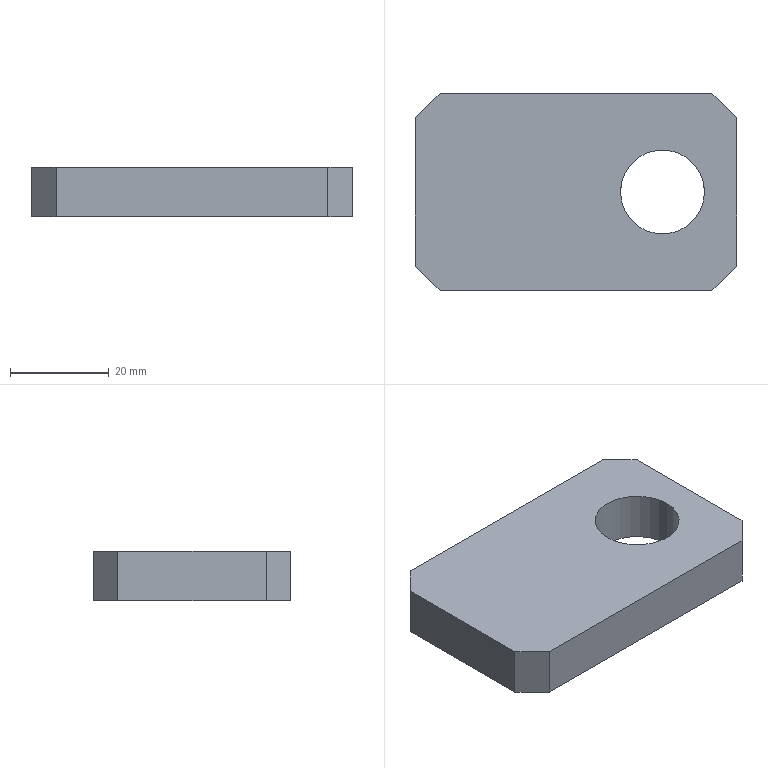Part | STEP file | BCC3 H12_2B | 1 solid | 12 faces | box 65 x 40 x 10 mm | volume 23230 mm3 | plane 10 | cylinder 2 | commonest cylinder face diameters 17 x2
STEP:
#1=CARTESIAN_POINT('',(0.,0.,0.));
#2=DIRECTION('',(0.,0.,1.));
#3=DIRECTION('',(1.,0.,0.));
#4=AXIS2_PLACEMENT_3D('',#1,#2,#3);
#5=CARTESIAN_POINT('',(9.,0.,5.));
#6=VERTEX_POINT('',#5);
#7=CARTESIAN_POINT('',(9.,0.,-5.));
#8=VERTEX_POINT('',#7);
#9=CARTESIAN_POINT('',(9.,0.,5.));
#10=DIRECTION('',(0.,0.,-1.));
#11=VECTOR('',#10,1.);
#12=LINE('',#9,#11);
#13=CARTESIAN_POINT('',(17.5,0.,5.));
#14=DIRECTION('',(0.,0.,-1.));
#15=DIRECTION('',(-1.,0.,0.));
#16=AXIS2_PLACEMENT_3D('',#13,#14,#15);
#17=CYLINDRICAL_SURFACE('',#16,8.5);
#18=CARTESIAN_POINT('',(6.283,0.));
#19=DIRECTION('',(0.,1.));
#20=VECTOR('',#19,1.);
#21=LINE('',#18,#20);
#22=(GEOMETRIC_REPRESENTATION_CONTEXT(2)PARAMETRIC_REPRESENTATION_CONTEXT()REPRESENTATION_CONTEXT('',''));
#23=DEFINITIONAL_REPRESENTATION('',(#21),#22);
#24=PCURVE('',#17,#23);
#25=CARTESIAN_POINT('',(17.5,0.,5.));
#26=DIRECTION('',(0.,0.,-1.));
#27=DIRECTION('',(-1.,0.,0.));
#28=AXIS2_PLACEMENT_3D('',#25,#26,#27);
#29=CYLINDRICAL_SURFACE('',#28,8.5);
#30=CARTESIAN_POINT('',(0.,0.));
#31=DIRECTION('',(0.,1.));
#32=VECTOR('',#31,1.);
#33=LINE('',#30,#32);
#34=(GEOMETRIC_REPRESENTATION_CONTEXT(2)PARAMETRIC_REPRESENTATION_CONTEXT()REPRESENTATION_CONTEXT('',''));
#35=DEFINITIONAL_REPRESENTATION('',(#33),#34);
#36=PCURVE('',#29,#35);
#37=SURFACE_CURVE('',#12,(#24,#36),.PCURVE_S1.);
#38=EDGE_CURVE('',#6,#8,#37,.T.);
#39=ORIENTED_EDGE('',*,*,#38,.T.);
#40=CARTESIAN_POINT('',(26.,0.,-5.));
#41=VERTEX_POINT('',#40);
#42=CARTESIAN_POINT('',(17.5,0.,-5.));
#43=DIRECTION('',(0.,0.,1.));
#44=DIRECTION('',(1.,0.,0.));
#45=AXIS2_PLACEMENT_3D('',#42,#43,#44);
#46=CIRCLE('',#45,8.5);
#47=CARTESIAN_POINT('',(9.425,10.));
#48=DIRECTION('',(-1.,0.));
#49=VECTOR('',#48,1.);
#50=LINE('',#47,#49);
#51=(GEOMETRIC_REPRESENTATION_CONTEXT(2)PARAMETRIC_REPRESENTATION_CONTEXT()REPRESENTATION_CONTEXT('',''));
#52=DEFINITIONAL_REPRESENTATION('',(#50),#51);
#53=PCURVE('',#17,#52);
#54=CARTESIAN_POINT('',(0.,0.,-5.));
#55=DIRECTION('',(0.,0.,1.));
#56=DIRECTION('',(1.,0.,0.));
#57=AXIS2_PLACEMENT_3D('',#54,#55,#56);
#58=PLANE('',#57);
#59=CARTESIAN_POINT('',(17.5,0.));
#60=DIRECTION('',(1.,0.));
#61=AXIS2_PLACEMENT_2D('',#59,#60);
#62=CIRCLE('',#61,8.5);
#63=(GEOMETRIC_REPRESENTATION_CONTEXT(2)PARAMETRIC_REPRESENTATION_CONTEXT()REPRESENTATION_CONTEXT('',''));
#64=DEFINITIONAL_REPRESENTATION('',(#62),#63);
#65=PCURVE('',#58,#64);
#66=SURFACE_CURVE('',#46,(#53,#65),.PCURVE_S1.);
#67=EDGE_CURVE('',#8,#41,#66,.T.);
#68=ORIENTED_EDGE('',*,*,#67,.T.);
#69=CARTESIAN_POINT('',(26.,0.,5.));
#70=VERTEX_POINT('',#69);
#71=CARTESIAN_POINT('',(26.,0.,5.));
#72=DIRECTION('',(0.,0.,-1.));
#73=VECTOR('',#72,1.);
#74=LINE('',#71,#73);
#75=CARTESIAN_POINT('',(3.142,0.));
#76=DIRECTION('',(0.,1.));
#77=VECTOR('',#76,1.);
#78=LINE('',#75,#77);
#79=(GEOMETRIC_REPRESENTATION_CONTEXT(2)PARAMETRIC_REPRESENTATION_CONTEXT()REPRESENTATION_CONTEXT('',''));
#80=DEFINITIONAL_REPRESENTATION('',(#78),#79);
#81=PCURVE('',#17,#80);
#82=CARTESIAN_POINT('',(3.142,0.));
#83=DIRECTION('',(0.,1.));
#84=VECTOR('',#83,1.);
#85=LINE('',#82,#84);
#86=(GEOMETRIC_REPRESENTATION_CONTEXT(2)PARAMETRIC_REPRESENTATION_CONTEXT()REPRESENTATION_CONTEXT('',''));
#87=DEFINITIONAL_REPRESENTATION('',(#85),#86);
#88=PCURVE('',#29,#87);
#89=SURFACE_CURVE('',#74,(#81,#88),.PCURVE_S1.);
#90=EDGE_CURVE('',#70,#41,#89,.T.);
#91=ORIENTED_EDGE('',*,*,#90,.F.);
#92=CARTESIAN_POINT('',(17.5,0.,5.));
#93=DIRECTION('',(0.,0.,1.));
#94=DIRECTION('',(1.,0.,0.));
#95=AXIS2_PLACEMENT_3D('',#92,#93,#94);
#96=CIRCLE('',#95,8.5);
#97=CARTESIAN_POINT('',(9.425,0.));
#98=DIRECTION('',(-1.,0.));
#99=VECTOR('',#98,1.);
#100=LINE('',#97,#99);
#101=(GEOMETRIC_REPRESENTATION_CONTEXT(2)PARAMETRIC_REPRESENTATION_CONTEXT()REPRESENTATION_CONTEXT('',''));
#102=DEFINITIONAL_REPRESENTATION('',(#100),#101);
#103=PCURVE('',#17,#102);
#104=CARTESIAN_POINT('',(0.,0.,5.));
#105=DIRECTION('',(0.,0.,1.));
#106=DIRECTION('',(1.,0.,0.));
#107=AXIS2_PLACEMENT_3D('',#104,#105,#106);
#108=PLANE('',#107);
#109=CARTESIAN_POINT('',(17.5,0.));
#110=DIRECTION('',(1.,0.));
#111=AXIS2_PLACEMENT_2D('',#109,#110);
#112=CIRCLE('',#111,8.5);
#113=(GEOMETRIC_REPRESENTATION_CONTEXT(2)PARAMETRIC_REPRESENTATION_CONTEXT()REPRESENTATION_CONTEXT('',''));
#114=DEFINITIONAL_REPRESENTATION('',(#112),#113);
#115=PCURVE('',#108,#114);
#116=SURFACE_CURVE('',#96,(#103,#115),.PCURVE_S1.);
#117=EDGE_CURVE('',#6,#70,#116,.T.);
#118=ORIENTED_EDGE('',*,*,#117,.F.);
#119=EDGE_LOOP('',(#39,#68,#91,#118));
#120=FACE_BOUND('',#119,.F.);
#121=ADVANCED_FACE('',(#120),#17,.F.);
#122=CARTESIAN_POINT('',(32.5,-15.,5.));
#123=VERTEX_POINT('',#122);
#124=CARTESIAN_POINT('',(32.5,15.,5.));
#125=VERTEX_POINT('',#124);
#126=CARTESIAN_POINT('',(32.5,20.,5.));
#127=DIRECTION('',(0.,1.,0.));
#128=VECTOR('',#127,1.);
#129=LINE('',#126,#128);
#130=CARTESIAN_POINT('',(32.5,20.));
#131=DIRECTION('',(0.,1.));
#132=VECTOR('',#131,1.);
#133=LINE('',#130,#132);
#134=(GEOMETRIC_REPRESENTATION_CONTEXT(2)PARAMETRIC_REPRESENTATION_CONTEXT()REPRESENTATION_CONTEXT('',''));
#135=DEFINITIONAL_REPRESENTATION('',(#133),#134);
#136=PCURVE('',#108,#135);
#137=CARTESIAN_POINT('',(32.5,20.,5.));
#138=DIRECTION('',(-1.,0.,0.));
#139=DIRECTION('',(0.,-1.,0.));
#140=AXIS2_PLACEMENT_3D('',#137,#138,#139);
#141=PLANE('',#140);
#142=CARTESIAN_POINT('',(0.,0.));
#143=DIRECTION('',(-1.,0.));
#144=VECTOR('',#143,1.);
#145=LINE('',#142,#144);
#146=(GEOMETRIC_REPRESENTATION_CONTEXT(2)PARAMETRIC_REPRESENTATION_CONTEXT()REPRESENTATION_CONTEXT('',''));
#147=DEFINITIONAL_REPRESENTATION('',(#145),#146);
#148=PCURVE('',#141,#147);
#149=SURFACE_CURVE('',#129,(#136,#148),.PCURVE_S1.);
#150=EDGE_CURVE('',#123,#125,#149,.T.);
#151=ORIENTED_EDGE('',*,*,#150,.T.);
#152=CARTESIAN_POINT('',(27.5,20.,5.));
#153=VERTEX_POINT('',#152);
#154=CARTESIAN_POINT('',(23.75,23.75,5.));
#155=DIRECTION('',(-0.7071,0.7071,0.));
#156=VECTOR('',#155,1.);
#157=LINE('',#154,#156);
#158=CARTESIAN_POINT('',(23.75,23.75));
#159=DIRECTION('',(-0.7071,0.7071));
#160=VECTOR('',#159,1.);
#161=LINE('',#158,#160);
#162=(GEOMETRIC_REPRESENTATION_CONTEXT(2)PARAMETRIC_REPRESENTATION_CONTEXT()REPRESENTATION_CONTEXT('',''));
#163=DEFINITIONAL_REPRESENTATION('',(#161),#162);
#164=PCURVE('',#108,#163);
#165=CARTESIAN_POINT('',(27.5,20.,5.));
#166=DIRECTION('',(-0.7071,-0.7071,0.));
#167=DIRECTION('',(0.,0.,-1.));
#168=AXIS2_PLACEMENT_3D('',#165,#166,#167);
#169=PLANE('',#168);
#170=CARTESIAN_POINT('',(0.,-5.303));
#171=DIRECTION('',(0.,-1.));
#172=VECTOR('',#171,1.);
#173=LINE('',#170,#172);
#174=(GEOMETRIC_REPRESENTATION_CONTEXT(2)PARAMETRIC_REPRESENTATION_CONTEXT()REPRESENTATION_CONTEXT('',''));
#175=DEFINITIONAL_REPRESENTATION('',(#173),#174);
#176=PCURVE('',#169,#175);
#177=SURFACE_CURVE('',#157,(#164,#176),.PCURVE_S1.);
#178=EDGE_CURVE('',#125,#153,#177,.T.);
#179=ORIENTED_EDGE('',*,*,#178,.T.);
#180=CARTESIAN_POINT('',(-27.5,20.,5.));
#181=VERTEX_POINT('',#180);
#182=CARTESIAN_POINT('',(-32.5,20.,5.));
#183=DIRECTION('',(-1.,0.,0.));
#184=VECTOR('',#183,1.);
#185=LINE('',#182,#184);
#186=CARTESIAN_POINT('',(-32.5,20.));
#187=DIRECTION('',(-1.,0.));
#188=VECTOR('',#187,1.);
#189=LINE('',#186,#188);
#190=(GEOMETRIC_REPRESENTATION_CONTEXT(2)PARAMETRIC_REPRESENTATION_CONTEXT()REPRESENTATION_CONTEXT('',''));
#191=DEFINITIONAL_REPRESENTATION('',(#189),#190);
#192=PCURVE('',#108,#191);
#193=CARTESIAN_POINT('',(-32.5,20.,5.));
#194=DIRECTION('',(0.,-1.,0.));
#195=DIRECTION('',(1.,0.,0.));
#196=AXIS2_PLACEMENT_3D('',#193,#194,#195);
#197=PLANE('',#196);
#198=CARTESIAN_POINT('',(0.,0.));
#199=DIRECTION('',(-1.,0.));
#200=VECTOR('',#199,1.);
#201=LINE('',#198,#200);
#202=(GEOMETRIC_REPRESENTATION_CONTEXT(2)PARAMETRIC_REPRESENTATION_CONTEXT()REPRESENTATION_CONTEXT('',''));
#203=DEFINITIONAL_REPRESENTATION('',(#201),#202);
#204=PCURVE('',#197,#203);
#205=SURFACE_CURVE('',#185,(#192,#204),.PCURVE_S1.);
#206=EDGE_CURVE('',#153,#181,#205,.T.);
#207=ORIENTED_EDGE('',*,*,#206,.T.);
#208=CARTESIAN_POINT('',(-32.5,15.,5.));
#209=VERTEX_POINT('',#208);
#210=CARTESIAN_POINT('',(-23.75,23.75,5.));
#211=DIRECTION('',(-0.7071,-0.7071,0.));
#212=VECTOR('',#211,1.);
#213=LINE('',#210,#212);
#214=CARTESIAN_POINT('',(-23.75,23.75));
#215=DIRECTION('',(-0.7071,-0.7071));
#216=VECTOR('',#215,1.);
#217=LINE('',#214,#216);
#218=(GEOMETRIC_REPRESENTATION_CONTEXT(2)PARAMETRIC_REPRESENTATION_CONTEXT()REPRESENTATION_CONTEXT('',''));
#219=DEFINITIONAL_REPRESENTATION('',(#217),#218);
#220=PCURVE('',#108,#219);
#221=CARTESIAN_POINT('',(-32.5,15.,5.));
#222=DIRECTION('',(0.7071,-0.7071,0.));
#223=DIRECTION('',(0.,0.,-1.));
#224=AXIS2_PLACEMENT_3D('',#221,#222,#223);
#225=PLANE('',#224);
#226=CARTESIAN_POINT('',(0.,12.374));
#227=DIRECTION('',(0.,-1.));
#228=VECTOR('',#227,1.);
#229=LINE('',#226,#228);
#230=(GEOMETRIC_REPRESENTATION_CONTEXT(2)PARAMETRIC_REPRESENTATION_CONTEXT()REPRESENTATION_CONTEXT('',''));
#231=DEFINITIONAL_REPRESENTATION('',(#229),#230);
#232=PCURVE('',#225,#231);
#233=SURFACE_CURVE('',#213,(#220,#232),.PCURVE_S1.);
#234=EDGE_CURVE('',#181,#209,#233,.T.);
#235=ORIENTED_EDGE('',*,*,#234,.T.);
#236=CARTESIAN_POINT('',(-32.5,-15.,5.));
#237=VERTEX_POINT('',#236);
#238=CARTESIAN_POINT('',(-32.5,20.,5.));
#239=DIRECTION('',(0.,-1.,0.));
#240=VECTOR('',#239,1.);
#241=LINE('',#238,#240);
#242=CARTESIAN_POINT('',(-32.5,20.));
#243=DIRECTION('',(0.,-1.));
#244=VECTOR('',#243,1.);
#245=LINE('',#242,#244);
#246=(GEOMETRIC_REPRESENTATION_CONTEXT(2)PARAMETRIC_REPRESENTATION_CONTEXT()REPRESENTATION_CONTEXT('',''));
#247=DEFINITIONAL_REPRESENTATION('',(#245),#246);
#248=PCURVE('',#108,#247);
#249=CARTESIAN_POINT('',(-32.5,20.,5.));
#250=DIRECTION('',(1.,0.,0.));
#251=DIRECTION('',(0.,1.,0.));
#252=AXIS2_PLACEMENT_3D('',#249,#250,#251);
#253=PLANE('',#252);
#254=CARTESIAN_POINT('',(0.,0.));
#255=DIRECTION('',(-1.,0.));
#256=VECTOR('',#255,1.);
#257=LINE('',#254,#256);
#258=(GEOMETRIC_REPRESENTATION_CONTEXT(2)PARAMETRIC_REPRESENTATION_CONTEXT()REPRESENTATION_CONTEXT('',''));
#259=DEFINITIONAL_REPRESENTATION('',(#257),#258);
#260=PCURVE('',#253,#259);
#261=SURFACE_CURVE('',#241,(#248,#260),.PCURVE_S1.);
#262=EDGE_CURVE('',#209,#237,#261,.T.);
#263=ORIENTED_EDGE('',*,*,#262,.T.);
#264=CARTESIAN_POINT('',(-27.5,-20.,5.));
#265=VERTEX_POINT('',#264);
#266=CARTESIAN_POINT('',(-23.75,-23.75,5.));
#267=DIRECTION('',(0.7071,-0.7071,0.));
#268=VECTOR('',#267,1.);
#269=LINE('',#266,#268);
#270=CARTESIAN_POINT('',(-23.75,-23.75));
#271=DIRECTION('',(0.7071,-0.7071));
#272=VECTOR('',#271,1.);
#273=LINE('',#270,#272);
#274=(GEOMETRIC_REPRESENTATION_CONTEXT(2)PARAMETRIC_REPRESENTATION_CONTEXT()REPRESENTATION_CONTEXT('',''));
#275=DEFINITIONAL_REPRESENTATION('',(#273),#274);
#276=PCURVE('',#108,#275);
#277=CARTESIAN_POINT('',(-27.5,-20.,5.));
#278=DIRECTION('',(0.7071,0.7071,0.));
#279=DIRECTION('',(0.,0.,-1.));
#280=AXIS2_PLACEMENT_3D('',#277,#278,#279);
#281=PLANE('',#280);
#282=CARTESIAN_POINT('',(0.,-5.303));
#283=DIRECTION('',(0.,-1.));
#284=VECTOR('',#283,1.);
#285=LINE('',#282,#284);
#286=(GEOMETRIC_REPRESENTATION_CONTEXT(2)PARAMETRIC_REPRESENTATION_CONTEXT()REPRESENTATION_CONTEXT('',''));
#287=DEFINITIONAL_REPRESENTATION('',(#285),#286);
#288=PCURVE('',#281,#287);
#289=SURFACE_CURVE('',#269,(#276,#288),.PCURVE_S1.);
#290=EDGE_CURVE('',#237,#265,#289,.T.);
#291=ORIENTED_EDGE('',*,*,#290,.T.);
#292=CARTESIAN_POINT('',(27.5,-20.,5.));
#293=VERTEX_POINT('',#292);
#294=CARTESIAN_POINT('',(-32.5,-20.,5.));
#295=DIRECTION('',(1.,0.,0.));
#296=VECTOR('',#295,1.);
#297=LINE('',#294,#296);
#298=CARTESIAN_POINT('',(-32.5,-20.));
#299=DIRECTION('',(1.,0.));
#300=VECTOR('',#299,1.);
#301=LINE('',#298,#300);
#302=(GEOMETRIC_REPRESENTATION_CONTEXT(2)PARAMETRIC_REPRESENTATION_CONTEXT()REPRESENTATION_CONTEXT('',''));
#303=DEFINITIONAL_REPRESENTATION('',(#301),#302);
#304=PCURVE('',#108,#303);
#305=CARTESIAN_POINT('',(-32.5,-20.,5.));
#306=DIRECTION('',(0.,1.,0.));
#307=DIRECTION('',(-1.,0.,0.));
#308=AXIS2_PLACEMENT_3D('',#305,#306,#307);
#309=PLANE('',#308);
#310=CARTESIAN_POINT('',(0.,0.));
#311=DIRECTION('',(-1.,0.));
#312=VECTOR('',#311,1.);
#313=LINE('',#310,#312);
#314=(GEOMETRIC_REPRESENTATION_CONTEXT(2)PARAMETRIC_REPRESENTATION_CONTEXT()REPRESENTATION_CONTEXT('',''));
#315=DEFINITIONAL_REPRESENTATION('',(#313),#314);
#316=PCURVE('',#309,#315);
#317=SURFACE_CURVE('',#297,(#304,#316),.PCURVE_S1.);
#318=EDGE_CURVE('',#265,#293,#317,.T.);
#319=ORIENTED_EDGE('',*,*,#318,.T.);
#320=CARTESIAN_POINT('',(23.75,-23.75,5.));
#321=DIRECTION('',(0.7071,0.7071,0.));
#322=VECTOR('',#321,1.);
#323=LINE('',#320,#322);
#324=CARTESIAN_POINT('',(23.75,-23.75));
#325=DIRECTION('',(0.7071,0.7071));
#326=VECTOR('',#325,1.);
#327=LINE('',#324,#326);
#328=(GEOMETRIC_REPRESENTATION_CONTEXT(2)PARAMETRIC_REPRESENTATION_CONTEXT()REPRESENTATION_CONTEXT('',''));
#329=DEFINITIONAL_REPRESENTATION('',(#327),#328);
#330=PCURVE('',#108,#329);
#331=CARTESIAN_POINT('',(32.5,-15.,5.));
#332=DIRECTION('',(-0.7071,0.7071,0.));
#333=DIRECTION('',(0.,0.,-1.));
#334=AXIS2_PLACEMENT_3D('',#331,#332,#333);
#335=PLANE('',#334);
#336=CARTESIAN_POINT('',(0.,12.374));
#337=DIRECTION('',(0.,-1.));
#338=VECTOR('',#337,1.);
#339=LINE('',#336,#338);
#340=(GEOMETRIC_REPRESENTATION_CONTEXT(2)PARAMETRIC_REPRESENTATION_CONTEXT()REPRESENTATION_CONTEXT('',''));
#341=DEFINITIONAL_REPRESENTATION('',(#339),#340);
#342=PCURVE('',#335,#341);
#343=SURFACE_CURVE('',#323,(#330,#342),.PCURVE_S1.);
#344=EDGE_CURVE('',#293,#123,#343,.T.);
#345=ORIENTED_EDGE('',*,*,#344,.T.);
#346=EDGE_LOOP('',(#151,#179,#207,#235,#263,#291,#319,#345));
#347=FACE_BOUND('',#346,.T.);
#348=ORIENTED_EDGE('',*,*,#117,.F.);
#349=CARTESIAN_POINT('',(17.5,0.,5.));
#350=DIRECTION('',(0.,0.,1.));
#351=DIRECTION('',(1.,0.,0.));
#352=AXIS2_PLACEMENT_3D('',#349,#350,#351);
#353=CIRCLE('',#352,8.5);
#354=CARTESIAN_POINT('',(17.5,0.));
#355=DIRECTION('',(1.,0.));
#356=AXIS2_PLACEMENT_2D('',#354,#355);
#357=CIRCLE('',#356,8.5);
#358=(GEOMETRIC_REPRESENTATION_CONTEXT(2)PARAMETRIC_REPRESENTATION_CONTEXT()REPRESENTATION_CONTEXT('',''));
#359=DEFINITIONAL_REPRESENTATION('',(#357),#358);
#360=PCURVE('',#108,#359);
#361=CARTESIAN_POINT('',(3.142,0.));
#362=DIRECTION('',(-1.,0.));
#363=VECTOR('',#362,1.);
#364=LINE('',#361,#363);
#365=(GEOMETRIC_REPRESENTATION_CONTEXT(2)PARAMETRIC_REPRESENTATION_CONTEXT()REPRESENTATION_CONTEXT('',''));
#366=DEFINITIONAL_REPRESENTATION('',(#364),#365);
#367=PCURVE('',#29,#366);
#368=SURFACE_CURVE('',#353,(#360,#367),.PCURVE_S1.);
#369=EDGE_CURVE('',#70,#6,#368,.T.);
#370=ORIENTED_EDGE('',*,*,#369,.F.);
#371=EDGE_LOOP('',(#348,#370));
#372=FACE_BOUND('',#371,.T.);
#373=ADVANCED_FACE('',(#347,#372),#108,.T.);
#374=CARTESIAN_POINT('',(27.5,20.,-5.));
#375=VERTEX_POINT('',#374);
#376=CARTESIAN_POINT('',(-27.5,20.,-5.));
#377=VERTEX_POINT('',#376);
#378=CARTESIAN_POINT('',(-32.5,20.,-5.));
#379=DIRECTION('',(-1.,0.,0.));
#380=VECTOR('',#379,1.);
#381=LINE('',#378,#380);
#382=CARTESIAN_POINT('',(-32.5,20.));
#383=DIRECTION('',(-1.,0.));
#384=VECTOR('',#383,1.);
#385=LINE('',#382,#384);
#386=(GEOMETRIC_REPRESENTATION_CONTEXT(2)PARAMETRIC_REPRESENTATION_CONTEXT()REPRESENTATION_CONTEXT('',''));
#387=DEFINITIONAL_REPRESENTATION('',(#385),#386);
#388=PCURVE('',#58,#387);
#389=CARTESIAN_POINT('',(0.,-10.));
#390=DIRECTION('',(-1.,0.));
#391=VECTOR('',#390,1.);
#392=LINE('',#389,#391);
#393=(GEOMETRIC_REPRESENTATION_CONTEXT(2)PARAMETRIC_REPRESENTATION_CONTEXT()REPRESENTATION_CONTEXT('',''));
#394=DEFINITIONAL_REPRESENTATION('',(#392),#393);
#395=PCURVE('',#197,#394);
#396=SURFACE_CURVE('',#381,(#388,#395),.PCURVE_S1.);
#397=EDGE_CURVE('',#375,#377,#396,.T.);
#398=ORIENTED_EDGE('',*,*,#397,.F.);
#399=CARTESIAN_POINT('',(32.5,15.,-5.));
#400=VERTEX_POINT('',#399);
#401=CARTESIAN_POINT('',(27.5,20.,-5.));
#402=DIRECTION('',(0.7071,-0.7071,0.));
#403=VECTOR('',#402,1.);
#404=LINE('',#401,#403);
#405=CARTESIAN_POINT('',(27.5,20.));
#406=DIRECTION('',(0.7071,-0.7071));
#407=VECTOR('',#406,1.);
#408=LINE('',#405,#407);
#409=(GEOMETRIC_REPRESENTATION_CONTEXT(2)PARAMETRIC_REPRESENTATION_CONTEXT()REPRESENTATION_CONTEXT('',''));
#410=DEFINITIONAL_REPRESENTATION('',(#408),#409);
#411=PCURVE('',#58,#410);
#412=CARTESIAN_POINT('',(10.,0.));
#413=DIRECTION('',(0.,1.));
#414=VECTOR('',#413,1.);
#415=LINE('',#412,#414);
#416=(GEOMETRIC_REPRESENTATION_CONTEXT(2)PARAMETRIC_REPRESENTATION_CONTEXT()REPRESENTATION_CONTEXT('',''));
#417=DEFINITIONAL_REPRESENTATION('',(#415),#416);
#418=PCURVE('',#169,#417);
#419=SURFACE_CURVE('',#404,(#411,#418),.PCURVE_S1.);
#420=EDGE_CURVE('',#375,#400,#419,.T.);
#421=ORIENTED_EDGE('',*,*,#420,.T.);
#422=CARTESIAN_POINT('',(32.5,-15.,-5.));
#423=VERTEX_POINT('',#422);
#424=CARTESIAN_POINT('',(32.5,20.,-5.));
#425=DIRECTION('',(0.,1.,0.));
#426=VECTOR('',#425,1.);
#427=LINE('',#424,#426);
#428=CARTESIAN_POINT('',(32.5,20.));
#429=DIRECTION('',(0.,1.));
#430=VECTOR('',#429,1.);
#431=LINE('',#428,#430);
#432=(GEOMETRIC_REPRESENTATION_CONTEXT(2)PARAMETRIC_REPRESENTATION_CONTEXT()REPRESENTATION_CONTEXT('',''));
#433=DEFINITIONAL_REPRESENTATION('',(#431),#432);
#434=PCURVE('',#58,#433);
#435=CARTESIAN_POINT('',(0.,-10.));
#436=DIRECTION('',(-1.,0.));
#437=VECTOR('',#436,1.);
#438=LINE('',#435,#437);
#439=(GEOMETRIC_REPRESENTATION_CONTEXT(2)PARAMETRIC_REPRESENTATION_CONTEXT()REPRESENTATION_CONTEXT('',''));
#440=DEFINITIONAL_REPRESENTATION('',(#438),#439);
#441=PCURVE('',#141,#440);
#442=SURFACE_CURVE('',#427,(#434,#441),.PCURVE_S1.);
#443=EDGE_CURVE('',#423,#400,#442,.T.);
#444=ORIENTED_EDGE('',*,*,#443,.F.);
#445=CARTESIAN_POINT('',(27.5,-20.,-5.));
#446=VERTEX_POINT('',#445);
#447=CARTESIAN_POINT('',(32.5,-15.,-5.));
#448=DIRECTION('',(-0.7071,-0.7071,0.));
#449=VECTOR('',#448,1.);
#450=LINE('',#447,#449);
#451=CARTESIAN_POINT('',(32.5,-15.));
#452=DIRECTION('',(-0.7071,-0.7071));
#453=VECTOR('',#452,1.);
#454=LINE('',#451,#453);
#455=(GEOMETRIC_REPRESENTATION_CONTEXT(2)PARAMETRIC_REPRESENTATION_CONTEXT()REPRESENTATION_CONTEXT('',''));
#456=DEFINITIONAL_REPRESENTATION('',(#454),#455);
#457=PCURVE('',#58,#456);
#458=CARTESIAN_POINT('',(10.,0.));
#459=DIRECTION('',(0.,1.));
#460=VECTOR('',#459,1.);
#461=LINE('',#458,#460);
#462=(GEOMETRIC_REPRESENTATION_CONTEXT(2)PARAMETRIC_REPRESENTATION_CONTEXT()REPRESENTATION_CONTEXT('',''));
#463=DEFINITIONAL_REPRESENTATION('',(#461),#462);
#464=PCURVE('',#335,#463);
#465=SURFACE_CURVE('',#450,(#457,#464),.PCURVE_S1.);
#466=EDGE_CURVE('',#423,#446,#465,.T.);
#467=ORIENTED_EDGE('',*,*,#466,.T.);
#468=CARTESIAN_POINT('',(-27.5,-20.,-5.));
#469=VERTEX_POINT('',#468);
#470=CARTESIAN_POINT('',(-32.5,-20.,-5.));
#471=DIRECTION('',(1.,0.,0.));
#472=VECTOR('',#471,1.);
#473=LINE('',#470,#472);
#474=CARTESIAN_POINT('',(-32.5,-20.));
#475=DIRECTION('',(1.,0.));
#476=VECTOR('',#475,1.);
#477=LINE('',#474,#476);
#478=(GEOMETRIC_REPRESENTATION_CONTEXT(2)PARAMETRIC_REPRESENTATION_CONTEXT()REPRESENTATION_CONTEXT('',''));
#479=DEFINITIONAL_REPRESENTATION('',(#477),#478);
#480=PCURVE('',#58,#479);
#481=CARTESIAN_POINT('',(0.,-10.));
#482=DIRECTION('',(-1.,0.));
#483=VECTOR('',#482,1.);
#484=LINE('',#481,#483);
#485=(GEOMETRIC_REPRESENTATION_CONTEXT(2)PARAMETRIC_REPRESENTATION_CONTEXT()REPRESENTATION_CONTEXT('',''));
#486=DEFINITIONAL_REPRESENTATION('',(#484),#485);
#487=PCURVE('',#309,#486);
#488=SURFACE_CURVE('',#473,(#480,#487),.PCURVE_S1.);
#489=EDGE_CURVE('',#469,#446,#488,.T.);
#490=ORIENTED_EDGE('',*,*,#489,.F.);
#491=CARTESIAN_POINT('',(-32.5,-15.,-5.));
#492=VERTEX_POINT('',#491);
#493=CARTESIAN_POINT('',(-27.5,-20.,-5.));
#494=DIRECTION('',(-0.7071,0.7071,0.));
#495=VECTOR('',#494,1.);
#496=LINE('',#493,#495);
#497=CARTESIAN_POINT('',(-27.5,-20.));
#498=DIRECTION('',(-0.7071,0.7071));
#499=VECTOR('',#498,1.);
#500=LINE('',#497,#499);
#501=(GEOMETRIC_REPRESENTATION_CONTEXT(2)PARAMETRIC_REPRESENTATION_CONTEXT()REPRESENTATION_CONTEXT('',''));
#502=DEFINITIONAL_REPRESENTATION('',(#500),#501);
#503=PCURVE('',#58,#502);
#504=CARTESIAN_POINT('',(10.,0.));
#505=DIRECTION('',(0.,1.));
#506=VECTOR('',#505,1.);
#507=LINE('',#504,#506);
#508=(GEOMETRIC_REPRESENTATION_CONTEXT(2)PARAMETRIC_REPRESENTATION_CONTEXT()REPRESENTATION_CONTEXT('',''));
#509=DEFINITIONAL_REPRESENTATION('',(#507),#508);
#510=PCURVE('',#281,#509);
#511=SURFACE_CURVE('',#496,(#503,#510),.PCURVE_S1.);
#512=EDGE_CURVE('',#469,#492,#511,.T.);
#513=ORIENTED_EDGE('',*,*,#512,.T.);
#514=CARTESIAN_POINT('',(-32.5,15.,-5.));
#515=VERTEX_POINT('',#514);
#516=CARTESIAN_POINT('',(-32.5,20.,-5.));
#517=DIRECTION('',(0.,-1.,0.));
#518=VECTOR('',#517,1.);
#519=LINE('',#516,#518);
#520=CARTESIAN_POINT('',(-32.5,20.));
#521=DIRECTION('',(0.,-1.));
#522=VECTOR('',#521,1.);
#523=LINE('',#520,#522);
#524=(GEOMETRIC_REPRESENTATION_CONTEXT(2)PARAMETRIC_REPRESENTATION_CONTEXT()REPRESENTATION_CONTEXT('',''));
#525=DEFINITIONAL_REPRESENTATION('',(#523),#524);
#526=PCURVE('',#58,#525);
#527=CARTESIAN_POINT('',(0.,-10.));
#528=DIRECTION('',(-1.,0.));
#529=VECTOR('',#528,1.);
#530=LINE('',#527,#529);
#531=(GEOMETRIC_REPRESENTATION_CONTEXT(2)PARAMETRIC_REPRESENTATION_CONTEXT()REPRESENTATION_CONTEXT('',''));
#532=DEFINITIONAL_REPRESENTATION('',(#530),#531);
#533=PCURVE('',#253,#532);
#534=SURFACE_CURVE('',#519,(#526,#533),.PCURVE_S1.);
#535=EDGE_CURVE('',#515,#492,#534,.T.);
#536=ORIENTED_EDGE('',*,*,#535,.F.);
#537=CARTESIAN_POINT('',(-32.5,15.,-5.));
#538=DIRECTION('',(0.7071,0.7071,0.));
#539=VECTOR('',#538,1.);
#540=LINE('',#537,#539);
#541=CARTESIAN_POINT('',(-32.5,15.));
#542=DIRECTION('',(0.7071,0.7071));
#543=VECTOR('',#542,1.);
#544=LINE('',#541,#543);
#545=(GEOMETRIC_REPRESENTATION_CONTEXT(2)PARAMETRIC_REPRESENTATION_CONTEXT()REPRESENTATION_CONTEXT('',''));
#546=DEFINITIONAL_REPRESENTATION('',(#544),#545);
#547=PCURVE('',#58,#546);
#548=CARTESIAN_POINT('',(10.,0.));
#549=DIRECTION('',(0.,1.));
#550=VECTOR('',#549,1.);
#551=LINE('',#548,#550);
#552=(GEOMETRIC_REPRESENTATION_CONTEXT(2)PARAMETRIC_REPRESENTATION_CONTEXT()REPRESENTATION_CONTEXT('',''));
#553=DEFINITIONAL_REPRESENTATION('',(#551),#552);
#554=PCURVE('',#225,#553);
#555=SURFACE_CURVE('',#540,(#547,#554),.PCURVE_S1.);
#556=EDGE_CURVE('',#515,#377,#555,.T.);
#557=ORIENTED_EDGE('',*,*,#556,.T.);
#558=EDGE_LOOP('',(#398,#421,#444,#467,#490,#513,#536,#557));
#559=FACE_BOUND('',#558,.T.);
#560=ORIENTED_EDGE('',*,*,#67,.T.);
#561=CARTESIAN_POINT('',(17.5,0.,-5.));
#562=DIRECTION('',(0.,0.,1.));
#563=DIRECTION('',(1.,0.,0.));
#564=AXIS2_PLACEMENT_3D('',#561,#562,#563);
#565=CIRCLE('',#564,8.5);
#566=CARTESIAN_POINT('',(17.5,0.));
#567=DIRECTION('',(1.,0.));
#568=AXIS2_PLACEMENT_2D('',#566,#567);
#569=CIRCLE('',#568,8.5);
#570=(GEOMETRIC_REPRESENTATION_CONTEXT(2)PARAMETRIC_REPRESENTATION_CONTEXT()REPRESENTATION_CONTEXT('',''));
#571=DEFINITIONAL_REPRESENTATION('',(#569),#570);
#572=PCURVE('',#58,#571);
#573=CARTESIAN_POINT('',(3.142,10.));
#574=DIRECTION('',(-1.,0.));
#575=VECTOR('',#574,1.);
#576=LINE('',#573,#575);
#577=(GEOMETRIC_REPRESENTATION_CONTEXT(2)PARAMETRIC_REPRESENTATION_CONTEXT()REPRESENTATION_CONTEXT('',''));
#578=DEFINITIONAL_REPRESENTATION('',(#576),#577);
#579=PCURVE('',#29,#578);
#580=SURFACE_CURVE('',#565,(#572,#579),.PCURVE_S1.);
#581=EDGE_CURVE('',#41,#8,#580,.T.);
#582=ORIENTED_EDGE('',*,*,#581,.T.);
#583=EDGE_LOOP('',(#560,#582));
#584=FACE_BOUND('',#583,.T.);
#585=ADVANCED_FACE('',(#559,#584),#58,.F.);
#586=ORIENTED_EDGE('',*,*,#535,.T.);
#587=CARTESIAN_POINT('',(-32.5,-15.,5.));
#588=DIRECTION('',(0.,0.,1.));
#589=VECTOR('',#588,1.);
#590=LINE('',#587,#589);
#591=CARTESIAN_POINT('',(-35.,0.));
#592=DIRECTION('',(0.,1.));
#593=VECTOR('',#592,1.);
#594=LINE('',#591,#593);
#595=(GEOMETRIC_REPRESENTATION_CONTEXT(2)PARAMETRIC_REPRESENTATION_CONTEXT()REPRESENTATION_CONTEXT('',''));
#596=DEFINITIONAL_REPRESENTATION('',(#594),#595);
#597=PCURVE('',#253,#596);
#598=CARTESIAN_POINT('',(0.,7.071));
#599=DIRECTION('',(-1.,0.));
#600=VECTOR('',#599,1.);
#601=LINE('',#598,#600);
#602=(GEOMETRIC_REPRESENTATION_CONTEXT(2)PARAMETRIC_REPRESENTATION_CONTEXT()REPRESENTATION_CONTEXT('',''));
#603=DEFINITIONAL_REPRESENTATION('',(#601),#602);
#604=PCURVE('',#281,#603);
#605=SURFACE_CURVE('',#590,(#597,#604),.PCURVE_S1.);
#606=EDGE_CURVE('',#492,#237,#605,.T.);
#607=ORIENTED_EDGE('',*,*,#606,.T.);
#608=ORIENTED_EDGE('',*,*,#262,.F.);
#609=CARTESIAN_POINT('',(-32.5,15.,5.));
#610=DIRECTION('',(0.,0.,-1.));
#611=VECTOR('',#610,1.);
#612=LINE('',#609,#611);
#613=CARTESIAN_POINT('',(-5.,0.));
#614=DIRECTION('',(0.,-1.));
#615=VECTOR('',#614,1.);
#616=LINE('',#613,#615);
#617=(GEOMETRIC_REPRESENTATION_CONTEXT(2)PARAMETRIC_REPRESENTATION_CONTEXT()REPRESENTATION_CONTEXT('',''));
#618=DEFINITIONAL_REPRESENTATION('',(#616),#617);
#619=PCURVE('',#253,#618);
#620=CARTESIAN_POINT('',(0.,0.));
#621=DIRECTION('',(1.,0.));
#622=VECTOR('',#621,1.);
#623=LINE('',#620,#622);
#624=(GEOMETRIC_REPRESENTATION_CONTEXT(2)PARAMETRIC_REPRESENTATION_CONTEXT()REPRESENTATION_CONTEXT('',''));
#625=DEFINITIONAL_REPRESENTATION('',(#623),#624);
#626=PCURVE('',#225,#625);
#627=SURFACE_CURVE('',#612,(#619,#626),.PCURVE_S1.);
#628=EDGE_CURVE('',#209,#515,#627,.T.);
#629=ORIENTED_EDGE('',*,*,#628,.T.);
#630=EDGE_LOOP('',(#586,#607,#608,#629));
#631=FACE_BOUND('',#630,.T.);
#632=ADVANCED_FACE('',(#631),#253,.F.);
#633=ORIENTED_EDGE('',*,*,#489,.T.);
#634=CARTESIAN_POINT('',(27.5,-20.,5.));
#635=DIRECTION('',(0.,0.,1.));
#636=VECTOR('',#635,1.);
#637=LINE('',#634,#636);
#638=CARTESIAN_POINT('',(-60.,0.));
#639=DIRECTION('',(0.,1.));
#640=VECTOR('',#639,1.);
#641=LINE('',#638,#640);
#642=(GEOMETRIC_REPRESENTATION_CONTEXT(2)PARAMETRIC_REPRESENTATION_CONTEXT()REPRESENTATION_CONTEXT('',''));
#643=DEFINITIONAL_REPRESENTATION('',(#641),#642);
#644=PCURVE('',#309,#643);
#645=CARTESIAN_POINT('',(0.,7.071));
#646=DIRECTION('',(-1.,0.));
#647=VECTOR('',#646,1.);
#648=LINE('',#645,#647);
#649=(GEOMETRIC_REPRESENTATION_CONTEXT(2)PARAMETRIC_REPRESENTATION_CONTEXT()REPRESENTATION_CONTEXT('',''));
#650=DEFINITIONAL_REPRESENTATION('',(#648),#649);
#651=PCURVE('',#335,#650);
#652=SURFACE_CURVE('',#637,(#644,#651),.PCURVE_S1.);
#653=EDGE_CURVE('',#446,#293,#652,.T.);
#654=ORIENTED_EDGE('',*,*,#653,.T.);
#655=ORIENTED_EDGE('',*,*,#318,.F.);
#656=CARTESIAN_POINT('',(-27.5,-20.,5.));
#657=DIRECTION('',(0.,0.,-1.));
#658=VECTOR('',#657,1.);
#659=LINE('',#656,#658);
#660=CARTESIAN_POINT('',(-5.,0.));
#661=DIRECTION('',(0.,-1.));
#662=VECTOR('',#661,1.);
#663=LINE('',#660,#662);
#664=(GEOMETRIC_REPRESENTATION_CONTEXT(2)PARAMETRIC_REPRESENTATION_CONTEXT()REPRESENTATION_CONTEXT('',''));
#665=DEFINITIONAL_REPRESENTATION('',(#663),#664);
#666=PCURVE('',#309,#665);
#667=CARTESIAN_POINT('',(0.,0.));
#668=DIRECTION('',(1.,0.));
#669=VECTOR('',#668,1.);
#670=LINE('',#667,#669);
#671=(GEOMETRIC_REPRESENTATION_CONTEXT(2)PARAMETRIC_REPRESENTATION_CONTEXT()REPRESENTATION_CONTEXT('',''));
#672=DEFINITIONAL_REPRESENTATION('',(#670),#671);
#673=PCURVE('',#281,#672);
#674=SURFACE_CURVE('',#659,(#666,#673),.PCURVE_S1.);
#675=EDGE_CURVE('',#265,#469,#674,.T.);
#676=ORIENTED_EDGE('',*,*,#675,.T.);
#677=EDGE_LOOP('',(#633,#654,#655,#676));
#678=FACE_BOUND('',#677,.T.);
#679=ADVANCED_FACE('',(#678),#309,.F.);
#680=ORIENTED_EDGE('',*,*,#443,.T.);
#681=CARTESIAN_POINT('',(32.5,15.,5.));
#682=DIRECTION('',(0.,0.,1.));
#683=VECTOR('',#682,1.);
#684=LINE('',#681,#683);
#685=CARTESIAN_POINT('',(5.,0.));
#686=DIRECTION('',(0.,1.));
#687=VECTOR('',#686,1.);
#688=LINE('',#685,#687);
#689=(GEOMETRIC_REPRESENTATION_CONTEXT(2)PARAMETRIC_REPRESENTATION_CONTEXT()REPRESENTATION_CONTEXT('',''));
#690=DEFINITIONAL_REPRESENTATION('',(#688),#689);
#691=PCURVE('',#141,#690);
#692=CARTESIAN_POINT('',(0.,7.071));
#693=DIRECTION('',(-1.,0.));
#694=VECTOR('',#693,1.);
#695=LINE('',#692,#694);
#696=(GEOMETRIC_REPRESENTATION_CONTEXT(2)PARAMETRIC_REPRESENTATION_CONTEXT()REPRESENTATION_CONTEXT('',''));
#697=DEFINITIONAL_REPRESENTATION('',(#695),#696);
#698=PCURVE('',#169,#697);
#699=SURFACE_CURVE('',#684,(#691,#698),.PCURVE_S1.);
#700=EDGE_CURVE('',#400,#125,#699,.T.);
#701=ORIENTED_EDGE('',*,*,#700,.T.);
#702=ORIENTED_EDGE('',*,*,#150,.F.);
#703=CARTESIAN_POINT('',(32.5,-15.,5.));
#704=DIRECTION('',(0.,0.,-1.));
#705=VECTOR('',#704,1.);
#706=LINE('',#703,#705);
#707=CARTESIAN_POINT('',(35.,0.));
#708=DIRECTION('',(0.,-1.));
#709=VECTOR('',#708,1.);
#710=LINE('',#707,#709);
#711=(GEOMETRIC_REPRESENTATION_CONTEXT(2)PARAMETRIC_REPRESENTATION_CONTEXT()REPRESENTATION_CONTEXT('',''));
#712=DEFINITIONAL_REPRESENTATION('',(#710),#711);
#713=PCURVE('',#141,#712);
#714=CARTESIAN_POINT('',(0.,0.));
#715=DIRECTION('',(1.,0.));
#716=VECTOR('',#715,1.);
#717=LINE('',#714,#716);
#718=(GEOMETRIC_REPRESENTATION_CONTEXT(2)PARAMETRIC_REPRESENTATION_CONTEXT()REPRESENTATION_CONTEXT('',''));
#719=DEFINITIONAL_REPRESENTATION('',(#717),#718);
#720=PCURVE('',#335,#719);
#721=SURFACE_CURVE('',#706,(#713,#720),.PCURVE_S1.);
#722=EDGE_CURVE('',#123,#423,#721,.T.);
#723=ORIENTED_EDGE('',*,*,#722,.T.);
#724=EDGE_LOOP('',(#680,#701,#702,#723));
#725=FACE_BOUND('',#724,.T.);
#726=ADVANCED_FACE('',(#725),#141,.F.);
#727=ORIENTED_EDGE('',*,*,#206,.F.);
#728=CARTESIAN_POINT('',(27.5,20.,5.));
#729=DIRECTION('',(0.,0.,-1.));
#730=VECTOR('',#729,1.);
#731=LINE('',#728,#730);
#732=CARTESIAN_POINT('',(60.,0.));
#733=DIRECTION('',(0.,-1.));
#734=VECTOR('',#733,1.);
#735=LINE('',#732,#734);
#736=(GEOMETRIC_REPRESENTATION_CONTEXT(2)PARAMETRIC_REPRESENTATION_CONTEXT()REPRESENTATION_CONTEXT('',''));
#737=DEFINITIONAL_REPRESENTATION('',(#735),#736);
#738=PCURVE('',#197,#737);
#739=CARTESIAN_POINT('',(0.,0.));
#740=DIRECTION('',(1.,0.));
#741=VECTOR('',#740,1.);
#742=LINE('',#739,#741);
#743=(GEOMETRIC_REPRESENTATION_CONTEXT(2)PARAMETRIC_REPRESENTATION_CONTEXT()REPRESENTATION_CONTEXT('',''));
#744=DEFINITIONAL_REPRESENTATION('',(#742),#743);
#745=PCURVE('',#169,#744);
#746=SURFACE_CURVE('',#731,(#738,#745),.PCURVE_S1.);
#747=EDGE_CURVE('',#153,#375,#746,.T.);
#748=ORIENTED_EDGE('',*,*,#747,.T.);
#749=ORIENTED_EDGE('',*,*,#397,.T.);
#750=CARTESIAN_POINT('',(-27.5,20.,5.));
#751=DIRECTION('',(0.,0.,1.));
#752=VECTOR('',#751,1.);
#753=LINE('',#750,#752);
#754=CARTESIAN_POINT('',(5.,0.));
#755=DIRECTION('',(0.,1.));
#756=VECTOR('',#755,1.);
#757=LINE('',#754,#756);
#758=(GEOMETRIC_REPRESENTATION_CONTEXT(2)PARAMETRIC_REPRESENTATION_CONTEXT()REPRESENTATION_CONTEXT('',''));
#759=DEFINITIONAL_REPRESENTATION('',(#757),#758);
#760=PCURVE('',#197,#759);
#761=CARTESIAN_POINT('',(0.,7.071));
#762=DIRECTION('',(-1.,0.));
#763=VECTOR('',#762,1.);
#764=LINE('',#761,#763);
#765=(GEOMETRIC_REPRESENTATION_CONTEXT(2)PARAMETRIC_REPRESENTATION_CONTEXT()REPRESENTATION_CONTEXT('',''));
#766=DEFINITIONAL_REPRESENTATION('',(#764),#765);
#767=PCURVE('',#225,#766);
#768=SURFACE_CURVE('',#753,(#760,#767),.PCURVE_S1.);
#769=EDGE_CURVE('',#377,#181,#768,.T.);
#770=ORIENTED_EDGE('',*,*,#769,.T.);
#771=EDGE_LOOP('',(#727,#748,#749,#770));
#772=FACE_BOUND('',#771,.T.);
#773=ADVANCED_FACE('',(#772),#197,.F.);
#774=ORIENTED_EDGE('',*,*,#581,.T.);
#775=ORIENTED_EDGE('',*,*,#38,.F.);
#776=ORIENTED_EDGE('',*,*,#369,.F.);
#777=ORIENTED_EDGE('',*,*,#90,.T.);
#778=EDGE_LOOP('',(#774,#775,#776,#777));
#779=FACE_BOUND('',#778,.F.);
#780=ADVANCED_FACE('',(#779),#29,.F.);
#781=ORIENTED_EDGE('',*,*,#178,.F.);
#782=ORIENTED_EDGE('',*,*,#700,.F.);
#783=ORIENTED_EDGE('',*,*,#420,.F.);
#784=ORIENTED_EDGE('',*,*,#747,.F.);
#785=EDGE_LOOP('',(#781,#782,#783,#784));
#786=FACE_BOUND('',#785,.T.);
#787=ADVANCED_FACE('',(#786),#169,.F.);
#788=ORIENTED_EDGE('',*,*,#344,.F.);
#789=ORIENTED_EDGE('',*,*,#653,.F.);
#790=ORIENTED_EDGE('',*,*,#466,.F.);
#791=ORIENTED_EDGE('',*,*,#722,.F.);
#792=EDGE_LOOP('',(#788,#789,#790,#791));
#793=FACE_BOUND('',#792,.T.);
#794=ADVANCED_FACE('',(#793),#335,.F.);
#795=ORIENTED_EDGE('',*,*,#290,.F.);
#796=ORIENTED_EDGE('',*,*,#606,.F.);
#797=ORIENTED_EDGE('',*,*,#512,.F.);
#798=ORIENTED_EDGE('',*,*,#675,.F.);
#799=EDGE_LOOP('',(#795,#796,#797,#798));
#800=FACE_BOUND('',#799,.T.);
#801=ADVANCED_FACE('',(#800),#281,.F.);
#802=ORIENTED_EDGE('',*,*,#234,.F.);
#803=ORIENTED_EDGE('',*,*,#769,.F.);
#804=ORIENTED_EDGE('',*,*,#556,.F.);
#805=ORIENTED_EDGE('',*,*,#628,.F.);
#806=EDGE_LOOP('',(#802,#803,#804,#805));
#807=FACE_BOUND('',#806,.T.);
#808=ADVANCED_FACE('',(#807),#225,.F.);
#809=CLOSED_SHELL('',(#121,#373,#585,#632,#679,#726,#773,#780,#787,#794,#801,#808));
#810=MANIFOLD_SOLID_BREP('',#809);
#811=(LENGTH_UNIT()NAMED_UNIT(*)SI_UNIT(.MILLI.,.METRE.));
#812=UNCERTAINTY_MEASURE_WITH_UNIT(LENGTH_MEASURE(0.0000001),#811,'','');
#813=(NAMED_UNIT(*)PLANE_ANGLE_UNIT()SI_UNIT($,.RADIAN.));
#814=(NAMED_UNIT(*)SI_UNIT($,.STERADIAN.)SOLID_ANGLE_UNIT());
#815=(GEOMETRIC_REPRESENTATION_CONTEXT(3)GLOBAL_UNCERTAINTY_ASSIGNED_CONTEXT((#812))GLOBAL_UNIT_ASSIGNED_CONTEXT((#811,#813,#814))REPRESENTATION_CONTEXT('',''));
#816=ADVANCED_BREP_SHAPE_REPRESENTATION('',(#4,#810),#815);